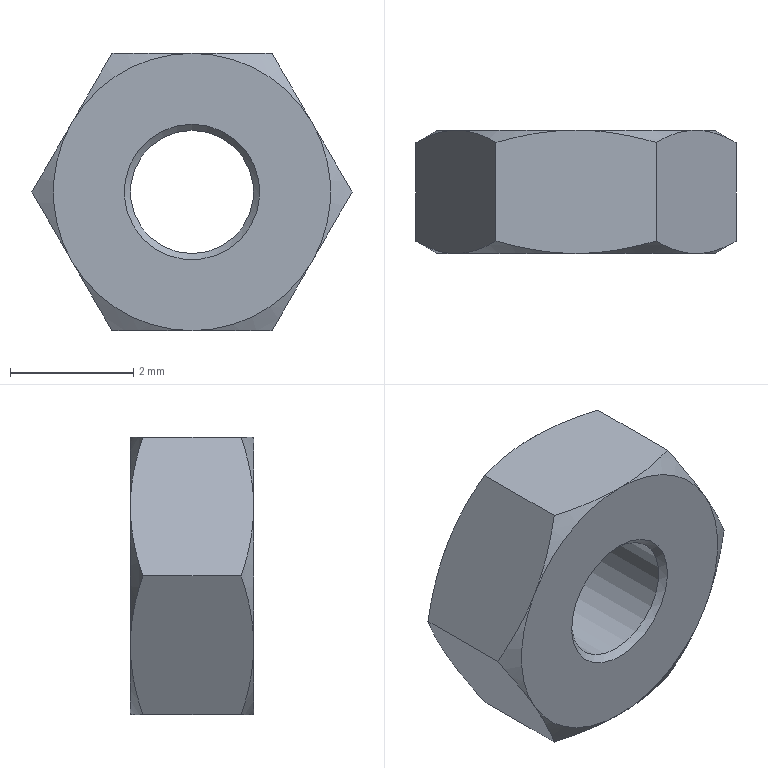Part | NX | features BREP 1 | 1 solid | 23 faces | box 5.196 x 2 x 4.5 mm | volume 28.526 mm3 | cone 14 | plane 8 | cylinder 1 | commonest cylinder face diameters 2 x1
STEP:
#1=CARTESIAN_POINT('',(0.,2.,1.1));
#2=VERTEX_POINT('',#1);
#3=CARTESIAN_POINT('',(0.,2.,0.));
#4=DIRECTION('',(0.,-1.,0.));
#5=DIRECTION('',(0.,0.,1.));
#6=AXIS2_PLACEMENT_3D('',#3,#4,#5);
#7=CIRCLE('',#6,1.1);
#8=EDGE_CURVE('',#2,#2,#7,.T.);
#9=ORIENTED_EDGE('',*,*,#8,.T.);
#10=EDGE_LOOP('',(#9));
#11=FACE_BOUND('',#10,.T.);
#12=CARTESIAN_POINT('',(-1.949,2.,1.125));
#13=VERTEX_POINT('',#12);
#14=CARTESIAN_POINT('',(0.,2.,2.25));
#15=VERTEX_POINT('',#14);
#16=CARTESIAN_POINT('',(0.,2.,0.));
#17=DIRECTION('',(0.,1.,0.));
#18=DIRECTION('',(0.,0.,1.));
#19=AXIS2_PLACEMENT_3D('',#16,#17,#18);
#20=CIRCLE('',#19,2.25);
#21=EDGE_CURVE('',#13,#15,#20,.T.);
#22=ORIENTED_EDGE('',*,*,#21,.T.);
#23=CARTESIAN_POINT('',(1.949,2.,1.125));
#24=VERTEX_POINT('',#23);
#25=CARTESIAN_POINT('',(0.,2.,0.));
#26=DIRECTION('',(0.,1.,0.));
#27=DIRECTION('',(0.,0.,1.));
#28=AXIS2_PLACEMENT_3D('',#25,#26,#27);
#29=CIRCLE('',#28,2.25);
#30=EDGE_CURVE('',#15,#24,#29,.T.);
#31=ORIENTED_EDGE('',*,*,#30,.T.);
#32=CARTESIAN_POINT('',(1.949,2.,-1.125));
#33=VERTEX_POINT('',#32);
#34=CARTESIAN_POINT('',(0.,2.,0.));
#35=DIRECTION('',(0.,1.,0.));
#36=DIRECTION('',(0.,0.,1.));
#37=AXIS2_PLACEMENT_3D('',#34,#35,#36);
#38=CIRCLE('',#37,2.25);
#39=EDGE_CURVE('',#24,#33,#38,.T.);
#40=ORIENTED_EDGE('',*,*,#39,.T.);
#41=CARTESIAN_POINT('',(0.,2.,-2.25));
#42=VERTEX_POINT('',#41);
#43=CARTESIAN_POINT('',(0.,2.,0.));
#44=DIRECTION('',(0.,1.,0.));
#45=DIRECTION('',(0.,0.,1.));
#46=AXIS2_PLACEMENT_3D('',#43,#44,#45);
#47=CIRCLE('',#46,2.25);
#48=EDGE_CURVE('',#33,#42,#47,.T.);
#49=ORIENTED_EDGE('',*,*,#48,.T.);
#50=CARTESIAN_POINT('',(-1.949,2.,-1.125));
#51=VERTEX_POINT('',#50);
#52=CARTESIAN_POINT('',(0.,2.,0.));
#53=DIRECTION('',(0.,1.,0.));
#54=DIRECTION('',(0.,0.,1.));
#55=AXIS2_PLACEMENT_3D('',#52,#53,#54);
#56=CIRCLE('',#55,2.25);
#57=EDGE_CURVE('',#42,#51,#56,.T.);
#58=ORIENTED_EDGE('',*,*,#57,.T.);
#59=CARTESIAN_POINT('',(0.,2.,0.));
#60=DIRECTION('',(0.,1.,0.));
#61=DIRECTION('',(0.,0.,1.));
#62=AXIS2_PLACEMENT_3D('',#59,#60,#61);
#63=CIRCLE('',#62,2.25);
#64=EDGE_CURVE('',#51,#13,#63,.T.);
#65=ORIENTED_EDGE('',*,*,#64,.T.);
#66=EDGE_LOOP('',(#22,#31,#40,#49,#58,#65));
#67=FACE_BOUND('',#66,.T.);
#68=CARTESIAN_POINT('',(0.,2.,0.));
#69=DIRECTION('',(0.,1.,0.));
#70=DIRECTION('',(0.,0.,-1.));
#71=AXIS2_PLACEMENT_3D('',#68,#69,#70);
#72=PLANE('',#71);
#73=ADVANCED_FACE('',(#11,#67),#72,.T.);
#74=CARTESIAN_POINT('',(1.299,1.799,2.25));
#75=VERTEX_POINT('',#74);
#76=CARTESIAN_POINT('',(1.299,1.799,2.25));
#77=CARTESIAN_POINT('',(1.511,1.922,1.882));
#78=CARTESIAN_POINT('',(1.727,2.,1.509));
#79=CARTESIAN_POINT('',(1.949,2.,1.125));
#80=B_SPLINE_CURVE_WITH_KNOTS('',3,(#76,#77,#78,#79),.UNSPECIFIED.,.F.,.F.,(4,4),(0.,0.001314),.UNSPECIFIED.);
#81=EDGE_CURVE('',#75,#24,#80,.T.);
#82=ORIENTED_EDGE('',*,*,#81,.F.);
#83=CARTESIAN_POINT('',(1.299,0.201,2.25));
#84=VERTEX_POINT('',#83);
#85=CARTESIAN_POINT('',(1.299,2.,2.25));
#86=DIRECTION('',(0.,-1.,0.));
#87=VECTOR('',#86,1000.);
#88=LINE('',#85,#87);
#89=EDGE_CURVE('',#75,#84,#88,.T.);
#90=ORIENTED_EDGE('',*,*,#89,.T.);
#91=CARTESIAN_POINT('',(1.949,0.,1.125));
#92=VERTEX_POINT('',#91);
#93=CARTESIAN_POINT('',(1.299,0.201,2.25));
#94=CARTESIAN_POINT('',(1.511,0.07844,1.882));
#95=CARTESIAN_POINT('',(1.727,0.,1.509));
#96=CARTESIAN_POINT('',(1.949,0.,1.125));
#97=B_SPLINE_CURVE_WITH_KNOTS('',3,(#93,#94,#95,#96),.UNSPECIFIED.,.F.,.F.,(4,4),(0.,0.001314),.UNSPECIFIED.);
#98=EDGE_CURVE('',#84,#92,#97,.T.);
#99=ORIENTED_EDGE('',*,*,#98,.T.);
#100=CARTESIAN_POINT('',(2.598,0.201,0.));
#101=VERTEX_POINT('',#100);
#102=CARTESIAN_POINT('',(1.949,0.,1.125));
#103=CARTESIAN_POINT('',(2.17,0.,0.741));
#104=CARTESIAN_POINT('',(2.386,0.07844,0.3676));
#105=CARTESIAN_POINT('',(2.598,0.201,0.));
#106=B_SPLINE_CURVE_WITH_KNOTS('',3,(#102,#103,#104,#105),.UNSPECIFIED.,.F.,.F.,(4,4),(0.,0.001314),.UNSPECIFIED.);
#107=EDGE_CURVE('',#92,#101,#106,.T.);
#108=ORIENTED_EDGE('',*,*,#107,.T.);
#109=CARTESIAN_POINT('',(2.598,1.799,0.));
#110=VERTEX_POINT('',#109);
#111=CARTESIAN_POINT('',(2.598,2.,0.));
#112=DIRECTION('',(0.,-1.,0.));
#113=VECTOR('',#112,1000.);
#114=LINE('',#111,#113);
#115=EDGE_CURVE('',#110,#101,#114,.T.);
#116=ORIENTED_EDGE('',*,*,#115,.F.);
#117=CARTESIAN_POINT('',(1.949,2.,1.125));
#118=CARTESIAN_POINT('',(2.17,2.,0.741));
#119=CARTESIAN_POINT('',(2.386,1.922,0.3676));
#120=CARTESIAN_POINT('',(2.598,1.799,0.));
#121=B_SPLINE_CURVE_WITH_KNOTS('',3,(#117,#118,#119,#120),.UNSPECIFIED.,.F.,.F.,(4,4),(0.,0.001314),.UNSPECIFIED.);
#122=EDGE_CURVE('',#24,#110,#121,.T.);
#123=ORIENTED_EDGE('',*,*,#122,.F.);
#124=EDGE_LOOP('',(#82,#90,#99,#108,#116,#123));
#125=FACE_BOUND('',#124,.T.);
#126=CARTESIAN_POINT('',(1.299,2.,2.25));
#127=DIRECTION('',(-0.866,0.,-0.5));
#128=DIRECTION('',(0.5,0.,-0.866));
#129=AXIS2_PLACEMENT_3D('',#126,#127,#128);
#130=PLANE('',#129);
#131=ADVANCED_FACE('',(#125),#130,.F.);
#132=CARTESIAN_POINT('',(2.598,1.799,0.));
#133=CARTESIAN_POINT('',(2.386,1.922,-0.3676));
#134=CARTESIAN_POINT('',(2.17,2.,-0.741));
#135=CARTESIAN_POINT('',(1.949,2.,-1.125));
#136=B_SPLINE_CURVE_WITH_KNOTS('',3,(#132,#133,#134,#135),.UNSPECIFIED.,.F.,.F.,(4,4),(0.,0.001314),.UNSPECIFIED.);
#137=EDGE_CURVE('',#110,#33,#136,.T.);
#138=ORIENTED_EDGE('',*,*,#137,.F.);
#139=ORIENTED_EDGE('',*,*,#115,.T.);
#140=CARTESIAN_POINT('',(1.949,0.,-1.125));
#141=VERTEX_POINT('',#140);
#142=CARTESIAN_POINT('',(2.598,0.201,0.));
#143=CARTESIAN_POINT('',(2.386,0.07844,-0.3676));
#144=CARTESIAN_POINT('',(2.17,0.,-0.741));
#145=CARTESIAN_POINT('',(1.949,0.,-1.125));
#146=B_SPLINE_CURVE_WITH_KNOTS('',3,(#142,#143,#144,#145),.UNSPECIFIED.,.F.,.F.,(4,4),(0.,0.001314),.UNSPECIFIED.);
#147=EDGE_CURVE('',#101,#141,#146,.T.);
#148=ORIENTED_EDGE('',*,*,#147,.T.);
#149=CARTESIAN_POINT('',(1.299,0.201,-2.25));
#150=VERTEX_POINT('',#149);
#151=CARTESIAN_POINT('',(1.949,0.,-1.125));
#152=CARTESIAN_POINT('',(1.727,0.,-1.509));
#153=CARTESIAN_POINT('',(1.511,0.07844,-1.882));
#154=CARTESIAN_POINT('',(1.299,0.201,-2.25));
#155=B_SPLINE_CURVE_WITH_KNOTS('',3,(#151,#152,#153,#154),.UNSPECIFIED.,.F.,.F.,(4,4),(0.,0.001314),.UNSPECIFIED.);
#156=EDGE_CURVE('',#141,#150,#155,.T.);
#157=ORIENTED_EDGE('',*,*,#156,.T.);
#158=CARTESIAN_POINT('',(1.299,1.799,-2.25));
#159=VERTEX_POINT('',#158);
#160=CARTESIAN_POINT('',(1.299,2.,-2.25));
#161=DIRECTION('',(0.,-1.,0.));
#162=VECTOR('',#161,1000.);
#163=LINE('',#160,#162);
#164=EDGE_CURVE('',#159,#150,#163,.T.);
#165=ORIENTED_EDGE('',*,*,#164,.F.);
#166=CARTESIAN_POINT('',(1.949,2.,-1.125));
#167=CARTESIAN_POINT('',(1.727,2.,-1.509));
#168=CARTESIAN_POINT('',(1.511,1.922,-1.882));
#169=CARTESIAN_POINT('',(1.299,1.799,-2.25));
#170=B_SPLINE_CURVE_WITH_KNOTS('',3,(#166,#167,#168,#169),.UNSPECIFIED.,.F.,.F.,(4,4),(0.,0.001314),.UNSPECIFIED.);
#171=EDGE_CURVE('',#33,#159,#170,.T.);
#172=ORIENTED_EDGE('',*,*,#171,.F.);
#173=EDGE_LOOP('',(#138,#139,#148,#157,#165,#172));
#174=FACE_BOUND('',#173,.T.);
#175=CARTESIAN_POINT('',(2.598,2.,0.));
#176=DIRECTION('',(-0.866,0.,0.5));
#177=DIRECTION('',(-0.5,0.,-0.866));
#178=AXIS2_PLACEMENT_3D('',#175,#176,#177);
#179=PLANE('',#178);
#180=ADVANCED_FACE('',(#174),#179,.F.);
#181=CARTESIAN_POINT('',(1.299,1.799,-2.25));
#182=CARTESIAN_POINT('',(0.8746,1.922,-2.25));
#183=CARTESIAN_POINT('',(0.4434,2.,-2.25));
#184=CARTESIAN_POINT('',(0.,2.,-2.25));
#185=B_SPLINE_CURVE_WITH_KNOTS('',3,(#181,#182,#183,#184),.UNSPECIFIED.,.F.,.F.,(4,4),(0.,0.001314),.UNSPECIFIED.);
#186=EDGE_CURVE('',#159,#42,#185,.T.);
#187=ORIENTED_EDGE('',*,*,#186,.F.);
#188=ORIENTED_EDGE('',*,*,#164,.T.);
#189=CARTESIAN_POINT('',(0.,0.,-2.25));
#190=VERTEX_POINT('',#189);
#191=CARTESIAN_POINT('',(1.299,0.201,-2.25));
#192=CARTESIAN_POINT('',(0.8746,0.07844,-2.25));
#193=CARTESIAN_POINT('',(0.4434,0.,-2.25));
#194=CARTESIAN_POINT('',(0.,0.,-2.25));
#195=B_SPLINE_CURVE_WITH_KNOTS('',3,(#191,#192,#193,#194),.UNSPECIFIED.,.F.,.F.,(4,4),(0.,0.001314),.UNSPECIFIED.);
#196=EDGE_CURVE('',#150,#190,#195,.T.);
#197=ORIENTED_EDGE('',*,*,#196,.T.);
#198=CARTESIAN_POINT('',(-1.299,0.201,-2.25));
#199=VERTEX_POINT('',#198);
#200=CARTESIAN_POINT('',(0.,0.,-2.25));
#201=CARTESIAN_POINT('',(-0.4434,0.,-2.25));
#202=CARTESIAN_POINT('',(-0.8746,0.07844,-2.25));
#203=CARTESIAN_POINT('',(-1.299,0.201,-2.25));
#204=B_SPLINE_CURVE_WITH_KNOTS('',3,(#200,#201,#202,#203),.UNSPECIFIED.,.F.,.F.,(4,4),(0.,0.001314),.UNSPECIFIED.);
#205=EDGE_CURVE('',#190,#199,#204,.T.);
#206=ORIENTED_EDGE('',*,*,#205,.T.);
#207=CARTESIAN_POINT('',(-1.299,1.799,-2.25));
#208=VERTEX_POINT('',#207);
#209=CARTESIAN_POINT('',(-1.299,2.,-2.25));
#210=DIRECTION('',(0.,-1.,0.));
#211=VECTOR('',#210,1000.);
#212=LINE('',#209,#211);
#213=EDGE_CURVE('',#208,#199,#212,.T.);
#214=ORIENTED_EDGE('',*,*,#213,.F.);
#215=CARTESIAN_POINT('',(0.,2.,-2.25));
#216=CARTESIAN_POINT('',(-0.4434,2.,-2.25));
#217=CARTESIAN_POINT('',(-0.8746,1.922,-2.25));
#218=CARTESIAN_POINT('',(-1.299,1.799,-2.25));
#219=B_SPLINE_CURVE_WITH_KNOTS('',3,(#215,#216,#217,#218),.UNSPECIFIED.,.F.,.F.,(4,4),(0.,0.001314),.UNSPECIFIED.);
#220=EDGE_CURVE('',#42,#208,#219,.T.);
#221=ORIENTED_EDGE('',*,*,#220,.F.);
#222=EDGE_LOOP('',(#187,#188,#197,#206,#214,#221));
#223=FACE_BOUND('',#222,.T.);
#224=CARTESIAN_POINT('',(1.299,2.,-2.25));
#225=DIRECTION('',(0.,0.,1.));
#226=DIRECTION('',(-1.,0.,0.));
#227=AXIS2_PLACEMENT_3D('',#224,#225,#226);
#228=PLANE('',#227);
#229=ADVANCED_FACE('',(#223),#228,.F.);
#230=CARTESIAN_POINT('',(-1.299,1.799,-2.25));
#231=CARTESIAN_POINT('',(-1.511,1.922,-1.882));
#232=CARTESIAN_POINT('',(-1.727,2.,-1.509));
#233=CARTESIAN_POINT('',(-1.949,2.,-1.125));
#234=B_SPLINE_CURVE_WITH_KNOTS('',3,(#230,#231,#232,#233),.UNSPECIFIED.,.F.,.F.,(4,4),(0.,0.001314),.UNSPECIFIED.);
#235=EDGE_CURVE('',#208,#51,#234,.T.);
#236=ORIENTED_EDGE('',*,*,#235,.F.);
#237=ORIENTED_EDGE('',*,*,#213,.T.);
#238=CARTESIAN_POINT('',(-1.949,0.,-1.125));
#239=VERTEX_POINT('',#238);
#240=CARTESIAN_POINT('',(-1.299,0.201,-2.25));
#241=CARTESIAN_POINT('',(-1.511,0.07844,-1.882));
#242=CARTESIAN_POINT('',(-1.727,0.,-1.509));
#243=CARTESIAN_POINT('',(-1.949,0.,-1.125));
#244=B_SPLINE_CURVE_WITH_KNOTS('',3,(#240,#241,#242,#243),.UNSPECIFIED.,.F.,.F.,(4,4),(0.,0.001314),.UNSPECIFIED.);
#245=EDGE_CURVE('',#199,#239,#244,.T.);
#246=ORIENTED_EDGE('',*,*,#245,.T.);
#247=CARTESIAN_POINT('',(-2.598,0.201,0.));
#248=VERTEX_POINT('',#247);
#249=CARTESIAN_POINT('',(-1.949,0.,-1.125));
#250=CARTESIAN_POINT('',(-2.17,0.,-0.741));
#251=CARTESIAN_POINT('',(-2.386,0.07844,-0.3676));
#252=CARTESIAN_POINT('',(-2.598,0.201,0.));
#253=B_SPLINE_CURVE_WITH_KNOTS('',3,(#249,#250,#251,#252),.UNSPECIFIED.,.F.,.F.,(4,4),(0.,0.001314),.UNSPECIFIED.);
#254=EDGE_CURVE('',#239,#248,#253,.T.);
#255=ORIENTED_EDGE('',*,*,#254,.T.);
#256=CARTESIAN_POINT('',(-2.598,1.799,0.));
#257=VERTEX_POINT('',#256);
#258=CARTESIAN_POINT('',(-2.598,2.,0.));
#259=DIRECTION('',(0.,-1.,0.));
#260=VECTOR('',#259,1000.);
#261=LINE('',#258,#260);
#262=EDGE_CURVE('',#257,#248,#261,.T.);
#263=ORIENTED_EDGE('',*,*,#262,.F.);
#264=CARTESIAN_POINT('',(-1.949,2.,-1.125));
#265=CARTESIAN_POINT('',(-2.17,2.,-0.741));
#266=CARTESIAN_POINT('',(-2.386,1.922,-0.3676));
#267=CARTESIAN_POINT('',(-2.598,1.799,0.));
#268=B_SPLINE_CURVE_WITH_KNOTS('',3,(#264,#265,#266,#267),.UNSPECIFIED.,.F.,.F.,(4,4),(0.,0.001314),.UNSPECIFIED.);
#269=EDGE_CURVE('',#51,#257,#268,.T.);
#270=ORIENTED_EDGE('',*,*,#269,.F.);
#271=EDGE_LOOP('',(#236,#237,#246,#255,#263,#270));
#272=FACE_BOUND('',#271,.T.);
#273=CARTESIAN_POINT('',(-1.299,2.,-2.25));
#274=DIRECTION('',(0.866,0.,0.5));
#275=DIRECTION('',(-0.5,0.,0.866));
#276=AXIS2_PLACEMENT_3D('',#273,#274,#275);
#277=PLANE('',#276);
#278=ADVANCED_FACE('',(#272),#277,.F.);
#279=CARTESIAN_POINT('',(-2.598,1.799,0.));
#280=CARTESIAN_POINT('',(-2.386,1.922,0.3676));
#281=CARTESIAN_POINT('',(-2.17,2.,0.741));
#282=CARTESIAN_POINT('',(-1.949,2.,1.125));
#283=B_SPLINE_CURVE_WITH_KNOTS('',3,(#279,#280,#281,#282),.UNSPECIFIED.,.F.,.F.,(4,4),(0.,0.001314),.UNSPECIFIED.);
#284=EDGE_CURVE('',#257,#13,#283,.T.);
#285=ORIENTED_EDGE('',*,*,#284,.F.);
#286=ORIENTED_EDGE('',*,*,#262,.T.);
#287=CARTESIAN_POINT('',(-1.949,0.,1.125));
#288=VERTEX_POINT('',#287);
#289=CARTESIAN_POINT('',(-2.598,0.201,0.));
#290=CARTESIAN_POINT('',(-2.386,0.07844,0.3676));
#291=CARTESIAN_POINT('',(-2.17,0.,0.741));
#292=CARTESIAN_POINT('',(-1.949,0.,1.125));
#293=B_SPLINE_CURVE_WITH_KNOTS('',3,(#289,#290,#291,#292),.UNSPECIFIED.,.F.,.F.,(4,4),(0.,0.001314),.UNSPECIFIED.);
#294=EDGE_CURVE('',#248,#288,#293,.T.);
#295=ORIENTED_EDGE('',*,*,#294,.T.);
#296=CARTESIAN_POINT('',(-1.299,0.201,2.25));
#297=VERTEX_POINT('',#296);
#298=CARTESIAN_POINT('',(-1.949,0.,1.125));
#299=CARTESIAN_POINT('',(-1.727,0.,1.509));
#300=CARTESIAN_POINT('',(-1.511,0.07844,1.882));
#301=CARTESIAN_POINT('',(-1.299,0.201,2.25));
#302=B_SPLINE_CURVE_WITH_KNOTS('',3,(#298,#299,#300,#301),.UNSPECIFIED.,.F.,.F.,(4,4),(0.,0.001314),.UNSPECIFIED.);
#303=EDGE_CURVE('',#288,#297,#302,.T.);
#304=ORIENTED_EDGE('',*,*,#303,.T.);
#305=CARTESIAN_POINT('',(-1.299,1.799,2.25));
#306=VERTEX_POINT('',#305);
#307=CARTESIAN_POINT('',(-1.299,2.,2.25));
#308=DIRECTION('',(0.,-1.,0.));
#309=VECTOR('',#308,1000.);
#310=LINE('',#307,#309);
#311=EDGE_CURVE('',#306,#297,#310,.T.);
#312=ORIENTED_EDGE('',*,*,#311,.F.);
#313=CARTESIAN_POINT('',(-1.949,2.,1.125));
#314=CARTESIAN_POINT('',(-1.727,2.,1.509));
#315=CARTESIAN_POINT('',(-1.511,1.922,1.882));
#316=CARTESIAN_POINT('',(-1.299,1.799,2.25));
#317=B_SPLINE_CURVE_WITH_KNOTS('',3,(#313,#314,#315,#316),.UNSPECIFIED.,.F.,.F.,(4,4),(0.,0.001314),.UNSPECIFIED.);
#318=EDGE_CURVE('',#13,#306,#317,.T.);
#319=ORIENTED_EDGE('',*,*,#318,.F.);
#320=EDGE_LOOP('',(#285,#286,#295,#304,#312,#319));
#321=FACE_BOUND('',#320,.T.);
#322=CARTESIAN_POINT('',(-2.598,2.,0.));
#323=DIRECTION('',(0.866,0.,-0.5));
#324=DIRECTION('',(0.5,0.,0.866));
#325=AXIS2_PLACEMENT_3D('',#322,#323,#324);
#326=PLANE('',#325);
#327=ADVANCED_FACE('',(#321),#326,.F.);
#328=CARTESIAN_POINT('',(-1.299,1.799,2.25));
#329=CARTESIAN_POINT('',(-0.8746,1.922,2.25));
#330=CARTESIAN_POINT('',(-0.4434,2.,2.25));
#331=CARTESIAN_POINT('',(0.,2.,2.25));
#332=B_SPLINE_CURVE_WITH_KNOTS('',3,(#328,#329,#330,#331),.UNSPECIFIED.,.F.,.F.,(4,4),(0.,0.001314),.UNSPECIFIED.);
#333=EDGE_CURVE('',#306,#15,#332,.T.);
#334=ORIENTED_EDGE('',*,*,#333,.F.);
#335=ORIENTED_EDGE('',*,*,#311,.T.);
#336=CARTESIAN_POINT('',(0.,0.,2.25));
#337=VERTEX_POINT('',#336);
#338=CARTESIAN_POINT('',(-1.299,0.201,2.25));
#339=CARTESIAN_POINT('',(-0.8746,0.07844,2.25));
#340=CARTESIAN_POINT('',(-0.4434,0.,2.25));
#341=CARTESIAN_POINT('',(0.,0.,2.25));
#342=B_SPLINE_CURVE_WITH_KNOTS('',3,(#338,#339,#340,#341),.UNSPECIFIED.,.F.,.F.,(4,4),(0.,0.001314),.UNSPECIFIED.);
#343=EDGE_CURVE('',#297,#337,#342,.T.);
#344=ORIENTED_EDGE('',*,*,#343,.T.);
#345=CARTESIAN_POINT('',(0.,0.,2.25));
#346=CARTESIAN_POINT('',(0.4434,0.,2.25));
#347=CARTESIAN_POINT('',(0.8746,0.07844,2.25));
#348=CARTESIAN_POINT('',(1.299,0.201,2.25));
#349=B_SPLINE_CURVE_WITH_KNOTS('',3,(#345,#346,#347,#348),.UNSPECIFIED.,.F.,.F.,(4,4),(0.,0.001314),.UNSPECIFIED.);
#350=EDGE_CURVE('',#337,#84,#349,.T.);
#351=ORIENTED_EDGE('',*,*,#350,.T.);
#352=ORIENTED_EDGE('',*,*,#89,.F.);
#353=CARTESIAN_POINT('',(0.,2.,2.25));
#354=CARTESIAN_POINT('',(0.4434,2.,2.25));
#355=CARTESIAN_POINT('',(0.8746,1.922,2.25));
#356=CARTESIAN_POINT('',(1.299,1.799,2.25));
#357=B_SPLINE_CURVE_WITH_KNOTS('',3,(#353,#354,#355,#356),.UNSPECIFIED.,.F.,.F.,(4,4),(0.,0.001314),.UNSPECIFIED.);
#358=EDGE_CURVE('',#15,#75,#357,.T.);
#359=ORIENTED_EDGE('',*,*,#358,.F.);
#360=EDGE_LOOP('',(#334,#335,#344,#351,#352,#359));
#361=FACE_BOUND('',#360,.T.);
#362=CARTESIAN_POINT('',(-1.299,2.,2.25));
#363=DIRECTION('',(0.,0.,-1.));
#364=DIRECTION('',(1.,0.,0.));
#365=AXIS2_PLACEMENT_3D('',#362,#363,#364);
#366=PLANE('',#365);
#367=ADVANCED_FACE('',(#361),#366,.F.);
#368=CARTESIAN_POINT('',(0.,0.,1.1));
#369=VERTEX_POINT('',#368);
#370=CARTESIAN_POINT('',(0.,0.,0.));
#371=DIRECTION('',(0.,1.,0.));
#372=DIRECTION('',(0.,0.,1.));
#373=AXIS2_PLACEMENT_3D('',#370,#371,#372);
#374=CIRCLE('',#373,1.1);
#375=EDGE_CURVE('',#369,#369,#374,.T.);
#376=ORIENTED_EDGE('',*,*,#375,.T.);
#377=EDGE_LOOP('',(#376));
#378=FACE_BOUND('',#377,.T.);
#379=CARTESIAN_POINT('',(0.,0.,0.));
#380=DIRECTION('',(0.,1.,0.));
#381=DIRECTION('',(0.,0.,1.));
#382=AXIS2_PLACEMENT_3D('',#379,#380,#381);
#383=CIRCLE('',#382,2.25);
#384=EDGE_CURVE('',#337,#92,#383,.T.);
#385=ORIENTED_EDGE('',*,*,#384,.F.);
#386=CARTESIAN_POINT('',(0.,0.,0.));
#387=DIRECTION('',(0.,1.,0.));
#388=DIRECTION('',(0.,0.,1.));
#389=AXIS2_PLACEMENT_3D('',#386,#387,#388);
#390=CIRCLE('',#389,2.25);
#391=EDGE_CURVE('',#288,#337,#390,.T.);
#392=ORIENTED_EDGE('',*,*,#391,.F.);
#393=CARTESIAN_POINT('',(0.,0.,0.));
#394=DIRECTION('',(0.,1.,0.));
#395=DIRECTION('',(0.,0.,1.));
#396=AXIS2_PLACEMENT_3D('',#393,#394,#395);
#397=CIRCLE('',#396,2.25);
#398=EDGE_CURVE('',#239,#288,#397,.T.);
#399=ORIENTED_EDGE('',*,*,#398,.F.);
#400=CARTESIAN_POINT('',(0.,0.,0.));
#401=DIRECTION('',(0.,1.,0.));
#402=DIRECTION('',(0.,0.,1.));
#403=AXIS2_PLACEMENT_3D('',#400,#401,#402);
#404=CIRCLE('',#403,2.25);
#405=EDGE_CURVE('',#190,#239,#404,.T.);
#406=ORIENTED_EDGE('',*,*,#405,.F.);
#407=CARTESIAN_POINT('',(0.,0.,0.));
#408=DIRECTION('',(0.,1.,0.));
#409=DIRECTION('',(0.,0.,1.));
#410=AXIS2_PLACEMENT_3D('',#407,#408,#409);
#411=CIRCLE('',#410,2.25);
#412=EDGE_CURVE('',#141,#190,#411,.T.);
#413=ORIENTED_EDGE('',*,*,#412,.F.);
#414=CARTESIAN_POINT('',(0.,0.,0.));
#415=DIRECTION('',(0.,1.,0.));
#416=DIRECTION('',(0.,0.,1.));
#417=AXIS2_PLACEMENT_3D('',#414,#415,#416);
#418=CIRCLE('',#417,2.25);
#419=EDGE_CURVE('',#92,#141,#418,.T.);
#420=ORIENTED_EDGE('',*,*,#419,.F.);
#421=EDGE_LOOP('',(#385,#392,#399,#406,#413,#420));
#422=FACE_BOUND('',#421,.T.);
#423=CARTESIAN_POINT('',(0.,0.,0.));
#424=DIRECTION('',(0.,1.,0.));
#425=DIRECTION('',(0.,0.,-1.));
#426=AXIS2_PLACEMENT_3D('',#423,#424,#425);
#427=PLANE('',#426);
#428=ADVANCED_FACE('',(#378,#422),#427,.F.);
#429=CARTESIAN_POINT('',(0.,0.1,1.));
#430=VERTEX_POINT('',#429);
#431=CARTESIAN_POINT('',(0.,0.1,0.));
#432=DIRECTION('',(0.,-1.,0.));
#433=DIRECTION('',(0.,0.,1.));
#434=AXIS2_PLACEMENT_3D('',#431,#432,#433);
#435=CIRCLE('',#434,1.);
#436=EDGE_CURVE('',#430,#430,#435,.T.);
#437=ORIENTED_EDGE('',*,*,#436,.T.);
#438=EDGE_LOOP('',(#437));
#439=FACE_BOUND('',#438,.T.);
#440=CARTESIAN_POINT('',(0.,1.9,1.));
#441=VERTEX_POINT('',#440);
#442=CARTESIAN_POINT('',(0.,1.9,0.));
#443=DIRECTION('',(0.,1.,0.));
#444=DIRECTION('',(0.,0.,1.));
#445=AXIS2_PLACEMENT_3D('',#442,#443,#444);
#446=CIRCLE('',#445,1.);
#447=EDGE_CURVE('',#441,#441,#446,.T.);
#448=ORIENTED_EDGE('',*,*,#447,.T.);
#449=EDGE_LOOP('',(#448));
#450=FACE_BOUND('',#449,.T.);
#451=CARTESIAN_POINT('',(0.,2.,0.));
#452=DIRECTION('',(0.,-1.,0.));
#453=DIRECTION('',(0.,0.,1.));
#454=AXIS2_PLACEMENT_3D('',#451,#452,#453);
#455=CYLINDRICAL_SURFACE('',#454,1.);
#456=ADVANCED_FACE('',(#439,#450),#455,.F.);
#457=ORIENTED_EDGE('',*,*,#350,.F.);
#458=ORIENTED_EDGE('',*,*,#384,.T.);
#459=ORIENTED_EDGE('',*,*,#98,.F.);
#460=EDGE_LOOP('',(#457,#458,#459));
#461=FACE_BOUND('',#460,.T.);
#462=CARTESIAN_POINT('',(0.,0.,0.));
#463=DIRECTION('',(0.,1.,0.));
#464=DIRECTION('',(0.,0.,-1.));
#465=AXIS2_PLACEMENT_3D('',#462,#463,#464);
#466=CONICAL_SURFACE('',#465,2.25,1.047);
#467=ADVANCED_FACE('',(#461),#466,.T.);
#468=ORIENTED_EDGE('',*,*,#391,.T.);
#469=ORIENTED_EDGE('',*,*,#343,.F.);
#470=ORIENTED_EDGE('',*,*,#303,.F.);
#471=EDGE_LOOP('',(#468,#469,#470));
#472=FACE_BOUND('',#471,.T.);
#473=CARTESIAN_POINT('',(0.,0.,0.));
#474=DIRECTION('',(0.,1.,0.));
#475=DIRECTION('',(0.,0.,-1.));
#476=AXIS2_PLACEMENT_3D('',#473,#474,#475);
#477=CONICAL_SURFACE('',#476,2.25,1.047);
#478=ADVANCED_FACE('',(#472),#477,.T.);
#479=ORIENTED_EDGE('',*,*,#398,.T.);
#480=ORIENTED_EDGE('',*,*,#294,.F.);
#481=ORIENTED_EDGE('',*,*,#254,.F.);
#482=EDGE_LOOP('',(#479,#480,#481));
#483=FACE_BOUND('',#482,.T.);
#484=CARTESIAN_POINT('',(0.,0.,0.));
#485=DIRECTION('',(0.,1.,0.));
#486=DIRECTION('',(0.,0.,-1.));
#487=AXIS2_PLACEMENT_3D('',#484,#485,#486);
#488=CONICAL_SURFACE('',#487,2.25,1.047);
#489=ADVANCED_FACE('',(#483),#488,.T.);
#490=ORIENTED_EDGE('',*,*,#405,.T.);
#491=ORIENTED_EDGE('',*,*,#245,.F.);
#492=ORIENTED_EDGE('',*,*,#205,.F.);
#493=EDGE_LOOP('',(#490,#491,#492));
#494=FACE_BOUND('',#493,.T.);
#495=CARTESIAN_POINT('',(0.,0.,0.));
#496=DIRECTION('',(0.,1.,0.));
#497=DIRECTION('',(0.,0.,-1.));
#498=AXIS2_PLACEMENT_3D('',#495,#496,#497);
#499=CONICAL_SURFACE('',#498,2.25,1.047);
#500=ADVANCED_FACE('',(#494),#499,.T.);
#501=ORIENTED_EDGE('',*,*,#412,.T.);
#502=ORIENTED_EDGE('',*,*,#196,.F.);
#503=ORIENTED_EDGE('',*,*,#156,.F.);
#504=EDGE_LOOP('',(#501,#502,#503));
#505=FACE_BOUND('',#504,.T.);
#506=CARTESIAN_POINT('',(0.,0.,0.));
#507=DIRECTION('',(0.,1.,0.));
#508=DIRECTION('',(0.,0.,-1.));
#509=AXIS2_PLACEMENT_3D('',#506,#507,#508);
#510=CONICAL_SURFACE('',#509,2.25,1.047);
#511=ADVANCED_FACE('',(#505),#510,.T.);
#512=ORIENTED_EDGE('',*,*,#419,.T.);
#513=ORIENTED_EDGE('',*,*,#147,.F.);
#514=ORIENTED_EDGE('',*,*,#107,.F.);
#515=EDGE_LOOP('',(#512,#513,#514));
#516=FACE_BOUND('',#515,.T.);
#517=CARTESIAN_POINT('',(0.,0.,0.));
#518=DIRECTION('',(0.,1.,0.));
#519=DIRECTION('',(0.,0.,-1.));
#520=AXIS2_PLACEMENT_3D('',#517,#518,#519);
#521=CONICAL_SURFACE('',#520,2.25,1.047);
#522=ADVANCED_FACE('',(#516),#521,.T.);
#523=ORIENTED_EDGE('',*,*,#81,.T.);
#524=ORIENTED_EDGE('',*,*,#30,.F.);
#525=ORIENTED_EDGE('',*,*,#358,.T.);
#526=EDGE_LOOP('',(#523,#524,#525));
#527=FACE_BOUND('',#526,.T.);
#528=CARTESIAN_POINT('',(0.,2.,0.));
#529=DIRECTION('',(0.,-1.,0.));
#530=DIRECTION('',(0.,0.,-1.));
#531=AXIS2_PLACEMENT_3D('',#528,#529,#530);
#532=CONICAL_SURFACE('',#531,2.25,1.047);
#533=ADVANCED_FACE('',(#527),#532,.T.);
#534=ORIENTED_EDGE('',*,*,#318,.T.);
#535=ORIENTED_EDGE('',*,*,#333,.T.);
#536=ORIENTED_EDGE('',*,*,#21,.F.);
#537=EDGE_LOOP('',(#534,#535,#536));
#538=FACE_BOUND('',#537,.T.);
#539=CARTESIAN_POINT('',(0.,2.,0.));
#540=DIRECTION('',(0.,-1.,0.));
#541=DIRECTION('',(0.,0.,-1.));
#542=AXIS2_PLACEMENT_3D('',#539,#540,#541);
#543=CONICAL_SURFACE('',#542,2.25,1.047);
#544=ADVANCED_FACE('',(#538),#543,.T.);
#545=ORIENTED_EDGE('',*,*,#269,.T.);
#546=ORIENTED_EDGE('',*,*,#284,.T.);
#547=ORIENTED_EDGE('',*,*,#64,.F.);
#548=EDGE_LOOP('',(#545,#546,#547));
#549=FACE_BOUND('',#548,.T.);
#550=CARTESIAN_POINT('',(0.,2.,0.));
#551=DIRECTION('',(0.,-1.,0.));
#552=DIRECTION('',(0.,0.,-1.));
#553=AXIS2_PLACEMENT_3D('',#550,#551,#552);
#554=CONICAL_SURFACE('',#553,2.25,1.047);
#555=ADVANCED_FACE('',(#549),#554,.T.);
#556=ORIENTED_EDGE('',*,*,#220,.T.);
#557=ORIENTED_EDGE('',*,*,#235,.T.);
#558=ORIENTED_EDGE('',*,*,#57,.F.);
#559=EDGE_LOOP('',(#556,#557,#558));
#560=FACE_BOUND('',#559,.T.);
#561=CARTESIAN_POINT('',(0.,2.,0.));
#562=DIRECTION('',(0.,-1.,0.));
#563=DIRECTION('',(0.,0.,-1.));
#564=AXIS2_PLACEMENT_3D('',#561,#562,#563);
#565=CONICAL_SURFACE('',#564,2.25,1.047);
#566=ADVANCED_FACE('',(#560),#565,.T.);
#567=ORIENTED_EDGE('',*,*,#171,.T.);
#568=ORIENTED_EDGE('',*,*,#186,.T.);
#569=ORIENTED_EDGE('',*,*,#48,.F.);
#570=EDGE_LOOP('',(#567,#568,#569));
#571=FACE_BOUND('',#570,.T.);
#572=CARTESIAN_POINT('',(0.,2.,0.));
#573=DIRECTION('',(0.,-1.,0.));
#574=DIRECTION('',(0.,0.,-1.));
#575=AXIS2_PLACEMENT_3D('',#572,#573,#574);
#576=CONICAL_SURFACE('',#575,2.25,1.047);
#577=ADVANCED_FACE('',(#571),#576,.T.);
#578=ORIENTED_EDGE('',*,*,#122,.T.);
#579=ORIENTED_EDGE('',*,*,#137,.T.);
#580=ORIENTED_EDGE('',*,*,#39,.F.);
#581=EDGE_LOOP('',(#578,#579,#580));
#582=FACE_BOUND('',#581,.T.);
#583=CARTESIAN_POINT('',(0.,2.,0.));
#584=DIRECTION('',(0.,-1.,0.));
#585=DIRECTION('',(0.,0.,-1.));
#586=AXIS2_PLACEMENT_3D('',#583,#584,#585);
#587=CONICAL_SURFACE('',#586,2.25,1.047);
#588=ADVANCED_FACE('',(#582),#587,.T.);
#589=ORIENTED_EDGE('',*,*,#436,.F.);
#590=EDGE_LOOP('',(#589));
#591=FACE_BOUND('',#590,.T.);
#592=ORIENTED_EDGE('',*,*,#375,.F.);
#593=EDGE_LOOP('',(#592));
#594=FACE_BOUND('',#593,.T.);
#595=CARTESIAN_POINT('',(0.,0.,0.));
#596=DIRECTION('',(0.,-1.,0.));
#597=DIRECTION('',(0.,0.,1.));
#598=AXIS2_PLACEMENT_3D('',#595,#596,#597);
#599=CONICAL_SURFACE('',#598,1.1,0.7854);
#600=ADVANCED_FACE('',(#591,#594),#599,.F.);
#601=ORIENTED_EDGE('',*,*,#8,.F.);
#602=EDGE_LOOP('',(#601));
#603=FACE_BOUND('',#602,.T.);
#604=ORIENTED_EDGE('',*,*,#447,.F.);
#605=EDGE_LOOP('',(#604));
#606=FACE_BOUND('',#605,.T.);
#607=CARTESIAN_POINT('',(0.,1.9,0.));
#608=DIRECTION('',(0.,1.,0.));
#609=DIRECTION('',(0.,0.,-1.));
#610=AXIS2_PLACEMENT_3D('',#607,#608,#609);
#611=CONICAL_SURFACE('',#610,1.,0.7854);
#612=ADVANCED_FACE('',(#603,#606),#611,.F.);
#613=CLOSED_SHELL('',(#73,#131,#180,#229,#278,#327,#367,#428,#456,#467,#478,#489,#500,#511,#522,#533,#544,#555,#566,#577,#588,#600,#612));
#614=MANIFOLD_SOLID_BREP('',#613);
#615=(LENGTH_UNIT()NAMED_UNIT(*)SI_UNIT(.MILLI.,.METRE.));
#616=UNCERTAINTY_MEASURE_WITH_UNIT(LENGTH_MEASURE(0.0508),#615,'','');
#617=(NAMED_UNIT(*)PLANE_ANGLE_UNIT()SI_UNIT($,.RADIAN.));
#618=(NAMED_UNIT(*)SI_UNIT($,.STERADIAN.)SOLID_ANGLE_UNIT());
#619=(GEOMETRIC_REPRESENTATION_CONTEXT(3)GLOBAL_UNCERTAINTY_ASSIGNED_CONTEXT((#616))GLOBAL_UNIT_ASSIGNED_CONTEXT((#615,#617,#618))REPRESENTATION_CONTEXT('',''));
#620=ADVANCED_BREP_SHAPE_REPRESENTATION('',(#614),#619);